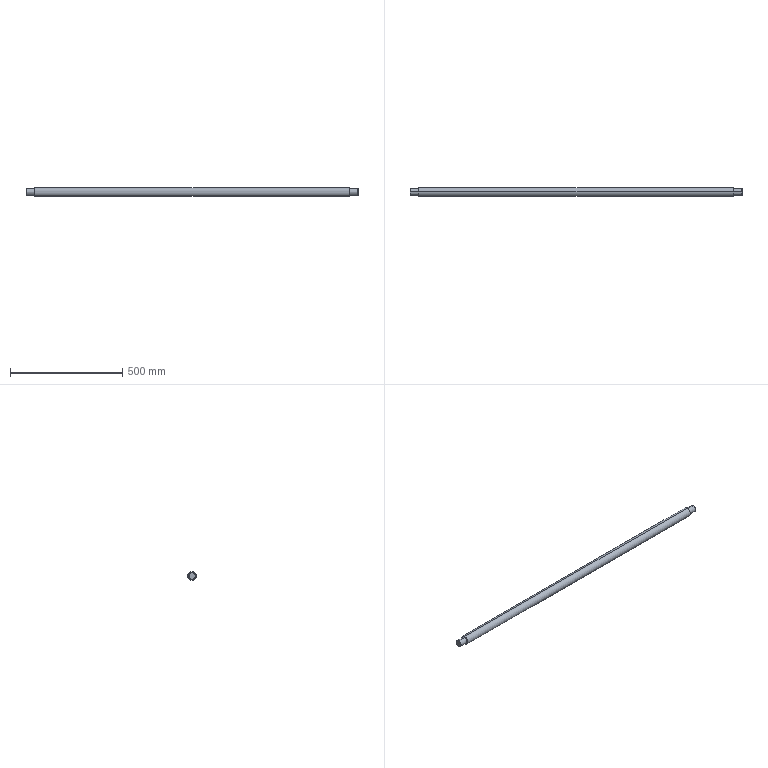Part | SolidWorks | features Chamfer 1, ICE 1, MirrorPattern 1, Revolution 1 | 1 solid | 29 faces | box 1476 x 40 x 40 mm | volume 1810594 mm3 | cone 10 | plane 10 | cylinder 9 | commonest cylinder face diameters 30 x4 8 x3 40 x2
STEP:
#1=CARTESIAN_POINT('',(-700.,0.,19.));
#2=VERTEX_POINT('',#1);
#3=CARTESIAN_POINT('',(-700.,0.,-19.));
#4=VERTEX_POINT('',#3);
#5=CARTESIAN_POINT('',(-700.,0.,0.));
#6=DIRECTION('',(-1.,0.,0.));
#7=DIRECTION('',(0.,0.,1.));
#8=AXIS2_PLACEMENT_3D('',#5,#6,#7);
#9=CIRCLE('',#8,19.);
#10=EDGE_CURVE('',#2,#4,#9,.T.);
#11=ORIENTED_EDGE('',*,*,#10,.F.);
#12=CARTESIAN_POINT('',(-699.,0.,20.));
#13=VERTEX_POINT('',#12);
#14=CARTESIAN_POINT('',(-699.,0.,20.));
#15=DIRECTION('',(0.7071,0.,0.7071));
#16=VECTOR('',#15,1000.);
#17=LINE('',#14,#16);
#18=EDGE_CURVE('',#2,#13,#17,.T.);
#19=ORIENTED_EDGE('',*,*,#18,.T.);
#20=CARTESIAN_POINT('',(-699.,0.,-20.));
#21=VERTEX_POINT('',#20);
#22=CARTESIAN_POINT('',(-699.,0.,0.));
#23=DIRECTION('',(1.,0.,0.));
#24=DIRECTION('',(0.,0.,1.));
#25=AXIS2_PLACEMENT_3D('',#22,#23,#24);
#26=CIRCLE('',#25,20.);
#27=EDGE_CURVE('',#21,#13,#26,.T.);
#28=ORIENTED_EDGE('',*,*,#27,.F.);
#29=CARTESIAN_POINT('',(-699.,0.,-20.));
#30=DIRECTION('',(0.7071,0.,-0.7071));
#31=VECTOR('',#30,1000.);
#32=LINE('',#29,#31);
#33=EDGE_CURVE('',#4,#21,#32,.T.);
#34=ORIENTED_EDGE('',*,*,#33,.F.);
#35=EDGE_LOOP('',(#11,#19,#28,#34));
#36=FACE_OUTER_BOUND('',#35,.T.);
#37=CARTESIAN_POINT('',(-699.,0.,0.));
#38=DIRECTION('',(1.,0.,0.));
#39=DIRECTION('',(0.,0.,-1.));
#40=AXIS2_PLACEMENT_3D('',#37,#38,#39);
#41=CONICAL_SURFACE('',#40,20.,0.7854);
#42=ADVANCED_FACE('',(#36),#41,.T.);
#43=CARTESIAN_POINT('',(-738.,0.,14.));
#44=VERTEX_POINT('',#43);
#45=CARTESIAN_POINT('',(-738.,13.416,4.));
#46=VERTEX_POINT('',#45);
#47=CARTESIAN_POINT('',(-738.,0.,0.));
#48=DIRECTION('',(-1.,0.,0.));
#49=DIRECTION('',(0.,0.,1.));
#50=AXIS2_PLACEMENT_3D('',#47,#48,#49);
#51=CIRCLE('',#50,14.);
#52=EDGE_CURVE('',#44,#46,#51,.T.);
#53=ORIENTED_EDGE('',*,*,#52,.F.);
#54=CARTESIAN_POINT('',(-737.,0.,15.));
#55=VERTEX_POINT('',#54);
#56=CARTESIAN_POINT('',(-737.,0.,15.));
#57=DIRECTION('',(0.7071,0.,0.7071));
#58=VECTOR('',#57,1000.);
#59=LINE('',#56,#58);
#60=EDGE_CURVE('',#44,#55,#59,.T.);
#61=ORIENTED_EDGE('',*,*,#60,.T.);
#62=CARTESIAN_POINT('',(-737.,14.457,4.));
#63=VERTEX_POINT('',#62);
#64=CARTESIAN_POINT('',(-737.,0.,0.));
#65=DIRECTION('',(1.,0.,0.));
#66=DIRECTION('',(0.,0.,1.));
#67=AXIS2_PLACEMENT_3D('',#64,#65,#66);
#68=CIRCLE('',#67,15.);
#69=EDGE_CURVE('',#63,#55,#68,.T.);
#70=ORIENTED_EDGE('',*,*,#69,.F.);
#71=CARTESIAN_POINT('',(-738.,13.416,4.));
#72=CARTESIAN_POINT('',(-737.667,13.764,4.));
#73=CARTESIAN_POINT('',(-737.334,14.11,4.));
#74=CARTESIAN_POINT('',(-737.,14.457,4.));
#75=B_SPLINE_CURVE_WITH_KNOTS('',3,(#71,#72,#73,#74),.UNSPECIFIED.,.F.,.F.,(4,4),(0.,0.001443),.UNSPECIFIED.);
#76=EDGE_CURVE('',#46,#63,#75,.T.);
#77=ORIENTED_EDGE('',*,*,#76,.F.);
#78=EDGE_LOOP('',(#53,#61,#70,#77));
#79=FACE_OUTER_BOUND('',#78,.T.);
#80=CARTESIAN_POINT('',(-737.,0.,0.));
#81=DIRECTION('',(1.,0.,0.));
#82=DIRECTION('',(0.,0.,-1.));
#83=AXIS2_PLACEMENT_3D('',#80,#81,#82);
#84=CONICAL_SURFACE('',#83,15.,0.7854);
#85=ADVANCED_FACE('',(#79),#84,.T.);
#86=ORIENTED_EDGE('',*,*,#60,.F.);
#87=CARTESIAN_POINT('',(-738.,0.,-14.));
#88=VERTEX_POINT('',#87);
#89=CARTESIAN_POINT('',(-738.,0.,0.));
#90=DIRECTION('',(-1.,0.,0.));
#91=DIRECTION('',(0.,0.,1.));
#92=AXIS2_PLACEMENT_3D('',#89,#90,#91);
#93=CIRCLE('',#92,14.);
#94=EDGE_CURVE('',#88,#44,#93,.T.);
#95=ORIENTED_EDGE('',*,*,#94,.F.);
#96=CARTESIAN_POINT('',(-737.,0.,-15.));
#97=VERTEX_POINT('',#96);
#98=CARTESIAN_POINT('',(-737.,0.,-15.));
#99=DIRECTION('',(0.7071,0.,-0.7071));
#100=VECTOR('',#99,1000.);
#101=LINE('',#98,#100);
#102=EDGE_CURVE('',#88,#97,#101,.T.);
#103=ORIENTED_EDGE('',*,*,#102,.T.);
#104=CARTESIAN_POINT('',(-737.,0.,0.));
#105=DIRECTION('',(1.,0.,0.));
#106=DIRECTION('',(0.,0.,1.));
#107=AXIS2_PLACEMENT_3D('',#104,#105,#106);
#108=CIRCLE('',#107,15.);
#109=EDGE_CURVE('',#55,#97,#108,.T.);
#110=ORIENTED_EDGE('',*,*,#109,.F.);
#111=EDGE_LOOP('',(#86,#95,#103,#110));
#112=FACE_OUTER_BOUND('',#111,.T.);
#113=CARTESIAN_POINT('',(-737.,0.,0.));
#114=DIRECTION('',(1.,0.,0.));
#115=DIRECTION('',(0.,0.,-1.));
#116=AXIS2_PLACEMENT_3D('',#113,#114,#115);
#117=CONICAL_SURFACE('',#116,15.,0.7854);
#118=ADVANCED_FACE('',(#112),#117,.T.);
#119=CARTESIAN_POINT('',(700.,0.,-19.));
#120=VERTEX_POINT('',#119);
#121=CARTESIAN_POINT('',(700.,0.,19.));
#122=VERTEX_POINT('',#121);
#123=CARTESIAN_POINT('',(700.,0.,0.));
#124=DIRECTION('',(1.,0.,0.));
#125=DIRECTION('',(0.,0.,-1.));
#126=AXIS2_PLACEMENT_3D('',#123,#124,#125);
#127=CIRCLE('',#126,19.);
#128=EDGE_CURVE('',#120,#122,#127,.T.);
#129=ORIENTED_EDGE('',*,*,#128,.F.);
#130=CARTESIAN_POINT('',(699.,0.,-20.));
#131=VERTEX_POINT('',#130);
#132=CARTESIAN_POINT('',(700.,0.,-19.));
#133=DIRECTION('',(-0.7071,0.,-0.7071));
#134=VECTOR('',#133,1000.);
#135=LINE('',#132,#134);
#136=EDGE_CURVE('',#120,#131,#135,.T.);
#137=ORIENTED_EDGE('',*,*,#136,.T.);
#138=CARTESIAN_POINT('',(699.,0.,20.));
#139=VERTEX_POINT('',#138);
#140=CARTESIAN_POINT('',(699.,0.,0.));
#141=DIRECTION('',(-1.,0.,0.));
#142=DIRECTION('',(0.,0.,-1.));
#143=AXIS2_PLACEMENT_3D('',#140,#141,#142);
#144=CIRCLE('',#143,20.);
#145=EDGE_CURVE('',#139,#131,#144,.T.);
#146=ORIENTED_EDGE('',*,*,#145,.F.);
#147=CARTESIAN_POINT('',(700.,0.,19.));
#148=DIRECTION('',(-0.7071,0.,0.7071));
#149=VECTOR('',#148,1000.);
#150=LINE('',#147,#149);
#151=EDGE_CURVE('',#122,#139,#150,.T.);
#152=ORIENTED_EDGE('',*,*,#151,.F.);
#153=EDGE_LOOP('',(#129,#137,#146,#152));
#154=FACE_OUTER_BOUND('',#153,.T.);
#155=CARTESIAN_POINT('',(700.,0.,0.));
#156=DIRECTION('',(-1.,0.,0.));
#157=DIRECTION('',(0.,0.,1.));
#158=AXIS2_PLACEMENT_3D('',#155,#156,#157);
#159=CONICAL_SURFACE('',#158,19.,0.7854);
#160=ADVANCED_FACE('',(#154),#159,.T.);
#161=CARTESIAN_POINT('',(738.,0.,-14.));
#162=VERTEX_POINT('',#161);
#163=CARTESIAN_POINT('',(738.,13.416,-4.));
#164=VERTEX_POINT('',#163);
#165=CARTESIAN_POINT('',(738.,0.,0.));
#166=DIRECTION('',(1.,0.,0.));
#167=DIRECTION('',(0.,0.,-1.));
#168=AXIS2_PLACEMENT_3D('',#165,#166,#167);
#169=CIRCLE('',#168,14.);
#170=EDGE_CURVE('',#162,#164,#169,.T.);
#171=ORIENTED_EDGE('',*,*,#170,.F.);
#172=CARTESIAN_POINT('',(737.,0.,-15.));
#173=VERTEX_POINT('',#172);
#174=CARTESIAN_POINT('',(738.,0.,-14.));
#175=DIRECTION('',(-0.7071,0.,-0.7071));
#176=VECTOR('',#175,1000.);
#177=LINE('',#174,#176);
#178=EDGE_CURVE('',#162,#173,#177,.T.);
#179=ORIENTED_EDGE('',*,*,#178,.T.);
#180=CARTESIAN_POINT('',(737.,14.457,-4.));
#181=VERTEX_POINT('',#180);
#182=CARTESIAN_POINT('',(737.,0.,0.));
#183=DIRECTION('',(-1.,0.,0.));
#184=DIRECTION('',(0.,0.,-1.));
#185=AXIS2_PLACEMENT_3D('',#182,#183,#184);
#186=CIRCLE('',#185,15.);
#187=EDGE_CURVE('',#181,#173,#186,.T.);
#188=ORIENTED_EDGE('',*,*,#187,.F.);
#189=CARTESIAN_POINT('',(738.,13.416,-4.));
#190=CARTESIAN_POINT('',(737.667,13.764,-4.));
#191=CARTESIAN_POINT('',(737.334,14.11,-4.));
#192=CARTESIAN_POINT('',(737.,14.457,-4.));
#193=B_SPLINE_CURVE_WITH_KNOTS('',3,(#189,#190,#191,#192),.UNSPECIFIED.,.F.,.F.,(4,4),(0.,0.001443),.UNSPECIFIED.);
#194=EDGE_CURVE('',#164,#181,#193,.T.);
#195=ORIENTED_EDGE('',*,*,#194,.F.);
#196=EDGE_LOOP('',(#171,#179,#188,#195));
#197=FACE_OUTER_BOUND('',#196,.T.);
#198=CARTESIAN_POINT('',(738.,0.,0.));
#199=DIRECTION('',(-1.,0.,0.));
#200=DIRECTION('',(0.,0.,1.));
#201=AXIS2_PLACEMENT_3D('',#198,#199,#200);
#202=CONICAL_SURFACE('',#201,14.,0.7854);
#203=ADVANCED_FACE('',(#197),#202,.T.);
#204=ORIENTED_EDGE('',*,*,#178,.F.);
#205=CARTESIAN_POINT('',(738.,0.,14.));
#206=VERTEX_POINT('',#205);
#207=CARTESIAN_POINT('',(738.,0.,0.));
#208=DIRECTION('',(1.,0.,0.));
#209=DIRECTION('',(0.,0.,-1.));
#210=AXIS2_PLACEMENT_3D('',#207,#208,#209);
#211=CIRCLE('',#210,14.);
#212=EDGE_CURVE('',#206,#162,#211,.T.);
#213=ORIENTED_EDGE('',*,*,#212,.F.);
#214=CARTESIAN_POINT('',(737.,0.,15.));
#215=VERTEX_POINT('',#214);
#216=CARTESIAN_POINT('',(738.,0.,14.));
#217=DIRECTION('',(-0.7071,0.,0.7071));
#218=VECTOR('',#217,1000.);
#219=LINE('',#216,#218);
#220=EDGE_CURVE('',#206,#215,#219,.T.);
#221=ORIENTED_EDGE('',*,*,#220,.T.);
#222=CARTESIAN_POINT('',(737.,0.,0.));
#223=DIRECTION('',(-1.,0.,0.));
#224=DIRECTION('',(0.,0.,-1.));
#225=AXIS2_PLACEMENT_3D('',#222,#223,#224);
#226=CIRCLE('',#225,15.);
#227=EDGE_CURVE('',#173,#215,#226,.T.);
#228=ORIENTED_EDGE('',*,*,#227,.F.);
#229=EDGE_LOOP('',(#204,#213,#221,#228));
#230=FACE_OUTER_BOUND('',#229,.T.);
#231=CARTESIAN_POINT('',(738.,0.,0.));
#232=DIRECTION('',(-1.,0.,0.));
#233=DIRECTION('',(0.,0.,1.));
#234=AXIS2_PLACEMENT_3D('',#231,#232,#233);
#235=CONICAL_SURFACE('',#234,14.,0.7854);
#236=ADVANCED_FACE('',(#230),#235,.T.);
#237=CARTESIAN_POINT('',(705.,11.,4.));
#238=VERTEX_POINT('',#237);
#239=CARTESIAN_POINT('',(701.,11.,0.));
#240=VERTEX_POINT('',#239);
#241=CARTESIAN_POINT('',(705.,11.,0.));
#242=DIRECTION('',(0.,-1.,0.));
#243=DIRECTION('',(1.,0.,0.));
#244=AXIS2_PLACEMENT_3D('',#241,#242,#243);
#245=CIRCLE('',#244,4.);
#246=EDGE_CURVE('',#238,#240,#245,.T.);
#247=ORIENTED_EDGE('',*,*,#246,.T.);
#248=CARTESIAN_POINT('',(701.,15.,0.));
#249=VERTEX_POINT('',#248);
#250=CARTESIAN_POINT('',(701.,11.,0.));
#251=DIRECTION('',(0.,1.,0.));
#252=VECTOR('',#251,1000.);
#253=LINE('',#250,#252);
#254=EDGE_CURVE('',#240,#249,#253,.T.);
#255=ORIENTED_EDGE('',*,*,#254,.T.);
#256=CARTESIAN_POINT('',(705.,14.457,4.));
#257=VERTEX_POINT('',#256);
#258=CARTESIAN_POINT('',(705.,14.457,4.));
#259=CARTESIAN_POINT('',(704.734,14.457,4.));
#260=CARTESIAN_POINT('',(704.473,14.464,3.974));
#261=CARTESIAN_POINT('',(703.96,14.492,3.871));
#262=CARTESIAN_POINT('',(703.706,14.513,3.794));
#263=CARTESIAN_POINT('',(703.222,14.564,3.593));
#264=CARTESIAN_POINT('',(702.992,14.594,3.47));
#265=CARTESIAN_POINT('',(702.558,14.66,3.179));
#266=CARTESIAN_POINT('',(702.354,14.696,3.011));
#267=CARTESIAN_POINT('',(701.987,14.766,2.644));
#268=CARTESIAN_POINT('',(701.822,14.801,2.443));
#269=CARTESIAN_POINT('',(701.529,14.867,2.006));
#270=CARTESIAN_POINT('',(701.406,14.897,1.775));
#271=CARTESIAN_POINT('',(701.206,14.946,1.293));
#272=CARTESIAN_POINT('',(701.129,14.966,1.04));
#273=CARTESIAN_POINT('',(701.026,14.993,0.5228));
#274=CARTESIAN_POINT('',(701.,15.,0.2623));
#275=CARTESIAN_POINT('',(701.,15.,0.));
#276=B_SPLINE_CURVE_WITH_KNOTS('',3,(#258,#259,#260,#261,#262,#263,#264,#265,#266,#267,#268,#269,#270,#271,#272,#273,#274,#275),.UNSPECIFIED.,.F.,.F.,(4,2,2,2,2,2,2,2,4),(0.,0.0007854,0.001571,0.002356,0.003142,0.003927,0.004712,0.005498,0.006283),.UNSPECIFIED.);
#277=EDGE_CURVE('',#257,#249,#276,.T.);
#278=ORIENTED_EDGE('',*,*,#277,.F.);
#279=CARTESIAN_POINT('',(705.,11.,4.));
#280=DIRECTION('',(0.,1.,0.));
#281=VECTOR('',#280,1000.);
#282=LINE('',#279,#281);
#283=EDGE_CURVE('',#238,#257,#282,.T.);
#284=ORIENTED_EDGE('',*,*,#283,.F.);
#285=EDGE_LOOP('',(#247,#255,#278,#284));
#286=FACE_OUTER_BOUND('',#285,.T.);
#287=CARTESIAN_POINT('',(705.,11.,0.));
#288=DIRECTION('',(0.,1.,0.));
#289=DIRECTION('',(-1.,0.,0.));
#290=AXIS2_PLACEMENT_3D('',#287,#288,#289);
#291=CYLINDRICAL_SURFACE('',#290,4.);
#292=ADVANCED_FACE('',(#286),#291,.F.);
#293=ORIENTED_EDGE('',*,*,#27,.T.);
#294=CARTESIAN_POINT('',(738.,0.,20.));
#295=DIRECTION('',(1.,0.,0.));
#296=VECTOR('',#295,1000.);
#297=LINE('',#294,#296);
#298=EDGE_CURVE('',#13,#139,#297,.T.);
#299=ORIENTED_EDGE('',*,*,#298,.T.);
#300=ORIENTED_EDGE('',*,*,#145,.T.);
#301=CARTESIAN_POINT('',(738.,0.,-20.));
#302=DIRECTION('',(1.,0.,0.));
#303=VECTOR('',#302,1000.);
#304=LINE('',#301,#303);
#305=EDGE_CURVE('',#21,#131,#304,.T.);
#306=ORIENTED_EDGE('',*,*,#305,.F.);
#307=EDGE_LOOP('',(#293,#299,#300,#306));
#308=FACE_OUTER_BOUND('',#307,.T.);
#309=CARTESIAN_POINT('',(738.,0.,0.));
#310=DIRECTION('',(1.,0.,0.));
#311=DIRECTION('',(0.,0.,-1.));
#312=AXIS2_PLACEMENT_3D('',#309,#310,#311);
#313=CYLINDRICAL_SURFACE('',#312,20.);
#314=ADVANCED_FACE('',(#308),#313,.T.);
#315=ORIENTED_EDGE('',*,*,#69,.T.);
#316=CARTESIAN_POINT('',(-700.,0.,15.));
#317=VERTEX_POINT('',#316);
#318=CARTESIAN_POINT('',(738.,0.,15.));
#319=DIRECTION('',(1.,0.,0.));
#320=VECTOR('',#319,1000.);
#321=LINE('',#318,#320);
#322=EDGE_CURVE('',#55,#317,#321,.T.);
#323=ORIENTED_EDGE('',*,*,#322,.T.);
#324=CARTESIAN_POINT('',(-700.,0.,-15.));
#325=VERTEX_POINT('',#324);
#326=CARTESIAN_POINT('',(-700.,0.,0.));
#327=DIRECTION('',(1.,0.,0.));
#328=DIRECTION('',(0.,0.,-1.));
#329=AXIS2_PLACEMENT_3D('',#326,#327,#328);
#330=CIRCLE('',#329,15.);
#331=EDGE_CURVE('',#325,#317,#330,.T.);
#332=ORIENTED_EDGE('',*,*,#331,.F.);
#333=CARTESIAN_POINT('',(738.,0.,-15.));
#334=DIRECTION('',(1.,0.,0.));
#335=VECTOR('',#334,1000.);
#336=LINE('',#333,#335);
#337=EDGE_CURVE('',#97,#325,#336,.T.);
#338=ORIENTED_EDGE('',*,*,#337,.F.);
#339=CARTESIAN_POINT('',(-737.,14.457,-4.));
#340=VERTEX_POINT('',#339);
#341=CARTESIAN_POINT('',(-737.,0.,0.));
#342=DIRECTION('',(1.,0.,0.));
#343=DIRECTION('',(0.,0.,1.));
#344=AXIS2_PLACEMENT_3D('',#341,#342,#343);
#345=CIRCLE('',#344,15.);
#346=EDGE_CURVE('',#97,#340,#345,.T.);
#347=ORIENTED_EDGE('',*,*,#346,.T.);
#348=CARTESIAN_POINT('',(-705.,14.457,-4.));
#349=VERTEX_POINT('',#348);
#350=CARTESIAN_POINT('',(738.,14.457,-4.));
#351=DIRECTION('',(-1.,0.,0.));
#352=VECTOR('',#351,1000.);
#353=LINE('',#350,#352);
#354=EDGE_CURVE('',#349,#340,#353,.T.);
#355=ORIENTED_EDGE('',*,*,#354,.F.);
#356=CARTESIAN_POINT('',(-705.,14.457,4.));
#357=VERTEX_POINT('',#356);
#358=CARTESIAN_POINT('',(-705.,14.457,4.));
#359=CARTESIAN_POINT('',(-704.734,14.457,4.));
#360=CARTESIAN_POINT('',(-704.474,14.464,3.974));
#361=CARTESIAN_POINT('',(-703.961,14.492,3.872));
#362=CARTESIAN_POINT('',(-703.706,14.513,3.794));
#363=CARTESIAN_POINT('',(-703.223,14.564,3.593));
#364=CARTESIAN_POINT('',(-702.993,14.594,3.47));
#365=CARTESIAN_POINT('',(-702.56,14.66,3.18));
#366=CARTESIAN_POINT('',(-702.355,14.696,3.012));
#367=CARTESIAN_POINT('',(-701.988,14.766,2.645));
#368=CARTESIAN_POINT('',(-701.823,14.801,2.444));
#369=CARTESIAN_POINT('',(-701.53,14.867,2.008));
#370=CARTESIAN_POINT('',(-701.407,14.896,1.777));
#371=CARTESIAN_POINT('',(-701.207,14.946,1.296));
#372=CARTESIAN_POINT('',(-701.129,14.966,1.043));
#373=CARTESIAN_POINT('',(-701.026,14.993,0.5261));
#374=CARTESIAN_POINT('',(-701.,15.,0.2658));
#375=CARTESIAN_POINT('',(-701.,15.,-0.2585));
#376=CARTESIAN_POINT('',(-701.026,14.993,-0.5249));
#377=CARTESIAN_POINT('',(-701.128,14.966,-1.039));
#378=CARTESIAN_POINT('',(-701.204,14.947,-1.289));
#379=CARTESIAN_POINT('',(-701.506,14.872,-2.017));
#380=CARTESIAN_POINT('',(-701.801,14.802,-2.457));
#381=CARTESIAN_POINT('',(-702.355,14.696,-3.012));
#382=CARTESIAN_POINT('',(-702.556,14.66,-3.177));
#383=CARTESIAN_POINT('',(-702.988,14.595,-3.467));
#384=CARTESIAN_POINT('',(-703.222,14.564,-3.593));
#385=CARTESIAN_POINT('',(-703.704,14.513,-3.793));
#386=CARTESIAN_POINT('',(-703.954,14.492,-3.87));
#387=CARTESIAN_POINT('',(-704.469,14.464,-3.973));
#388=CARTESIAN_POINT('',(-704.734,14.457,-4.));
#389=CARTESIAN_POINT('',(-705.,14.457,-4.));
#390=B_SPLINE_CURVE_WITH_KNOTS('',3,(#358,#359,#360,#361,#362,#363,#364,#365,#366,#367,#368,#369,#370,#371,#372,#373,#374,#375,#376,#377,#378,#379,#380,#381,#382,#383,#384,#385,#386,#387,#388,#389),.UNSPECIFIED.,.F.,.F.,(4,2,2,2,2,2,2,2,2,2,2,2,2,2,2,4),(0.,0.0007849,0.00157,0.002355,0.00314,0.003925,0.00471,0.005494,0.006279,0.007064,0.007849,0.009419,0.0102,0.01099,0.01177,0.01256),.UNSPECIFIED.);
#391=EDGE_CURVE('',#357,#349,#390,.T.);
#392=ORIENTED_EDGE('',*,*,#391,.F.);
#393=CARTESIAN_POINT('',(738.,14.457,4.));
#394=DIRECTION('',(1.,0.,0.));
#395=VECTOR('',#394,1000.);
#396=LINE('',#393,#395);
#397=EDGE_CURVE('',#63,#357,#396,.T.);
#398=ORIENTED_EDGE('',*,*,#397,.F.);
#399=EDGE_LOOP('',(#315,#323,#332,#338,#347,#355,#392,#398));
#400=FACE_OUTER_BOUND('',#399,.T.);
#401=CARTESIAN_POINT('',(738.,0.,0.));
#402=DIRECTION('',(1.,0.,0.));
#403=DIRECTION('',(0.,0.,-1.));
#404=AXIS2_PLACEMENT_3D('',#401,#402,#403);
#405=CYLINDRICAL_SURFACE('',#404,15.);
#406=ADVANCED_FACE('',(#400),#405,.T.);
#407=CARTESIAN_POINT('',(700.,0.,-15.));
#408=VERTEX_POINT('',#407);
#409=CARTESIAN_POINT('',(700.,0.,15.));
#410=VERTEX_POINT('',#409);
#411=CARTESIAN_POINT('',(700.,0.,0.));
#412=DIRECTION('',(1.,0.,0.));
#413=DIRECTION('',(0.,0.,-1.));
#414=AXIS2_PLACEMENT_3D('',#411,#412,#413);
#415=CIRCLE('',#414,15.);
#416=EDGE_CURVE('',#408,#410,#415,.T.);
#417=ORIENTED_EDGE('',*,*,#416,.T.);
#418=CARTESIAN_POINT('',(738.,0.,15.));
#419=DIRECTION('',(1.,0.,0.));
#420=VECTOR('',#419,1000.);
#421=LINE('',#418,#420);
#422=EDGE_CURVE('',#410,#215,#421,.T.);
#423=ORIENTED_EDGE('',*,*,#422,.T.);
#424=CARTESIAN_POINT('',(737.,14.457,4.));
#425=VERTEX_POINT('',#424);
#426=CARTESIAN_POINT('',(737.,0.,0.));
#427=DIRECTION('',(-1.,0.,0.));
#428=DIRECTION('',(0.,0.,-1.));
#429=AXIS2_PLACEMENT_3D('',#426,#427,#428);
#430=CIRCLE('',#429,15.);
#431=EDGE_CURVE('',#215,#425,#430,.T.);
#432=ORIENTED_EDGE('',*,*,#431,.T.);
#433=CARTESIAN_POINT('',(738.,14.457,4.));
#434=DIRECTION('',(-1.,0.,0.));
#435=VECTOR('',#434,1000.);
#436=LINE('',#433,#435);
#437=EDGE_CURVE('',#425,#257,#436,.T.);
#438=ORIENTED_EDGE('',*,*,#437,.T.);
#439=ORIENTED_EDGE('',*,*,#277,.T.);
#440=CARTESIAN_POINT('',(705.,14.457,-4.));
#441=VERTEX_POINT('',#440);
#442=CARTESIAN_POINT('',(701.,15.,0.));
#443=CARTESIAN_POINT('',(701.,15.,-0.262));
#444=CARTESIAN_POINT('',(701.026,14.993,-0.5282));
#445=CARTESIAN_POINT('',(701.129,14.966,-1.042));
#446=CARTESIAN_POINT('',(701.205,14.946,-1.292));
#447=CARTESIAN_POINT('',(701.508,14.871,-2.02));
#448=CARTESIAN_POINT('',(701.802,14.802,-2.459));
#449=CARTESIAN_POINT('',(702.357,14.695,-3.014));
#450=CARTESIAN_POINT('',(702.557,14.66,-3.178));
#451=CARTESIAN_POINT('',(702.989,14.594,-3.467));
#452=CARTESIAN_POINT('',(703.223,14.564,-3.593));
#453=CARTESIAN_POINT('',(703.705,14.513,-3.794));
#454=CARTESIAN_POINT('',(703.954,14.492,-3.87));
#455=CARTESIAN_POINT('',(704.469,14.464,-3.973));
#456=CARTESIAN_POINT('',(704.735,14.457,-4.));
#457=CARTESIAN_POINT('',(705.,14.457,-4.));
#458=B_SPLINE_CURVE_WITH_KNOTS('',3,(#442,#443,#444,#445,#446,#447,#448,#449,#450,#451,#452,#453,#454,#455,#456,#457),.UNSPECIFIED.,.F.,.F.,(4,2,2,2,2,2,2,4),(0.006283,0.007068,0.007852,0.009421,0.01021,0.01099,0.01177,0.01256),.UNSPECIFIED.);
#459=EDGE_CURVE('',#249,#441,#458,.T.);
#460=ORIENTED_EDGE('',*,*,#459,.T.);
#461=CARTESIAN_POINT('',(738.,14.457,-4.));
#462=DIRECTION('',(1.,0.,0.));
#463=VECTOR('',#462,1000.);
#464=LINE('',#461,#463);
#465=EDGE_CURVE('',#441,#181,#464,.T.);
#466=ORIENTED_EDGE('',*,*,#465,.T.);
#467=ORIENTED_EDGE('',*,*,#187,.T.);
#468=CARTESIAN_POINT('',(738.,0.,-15.));
#469=DIRECTION('',(1.,0.,0.));
#470=VECTOR('',#469,1000.);
#471=LINE('',#468,#470);
#472=EDGE_CURVE('',#408,#173,#471,.T.);
#473=ORIENTED_EDGE('',*,*,#472,.F.);
#474=EDGE_LOOP('',(#417,#423,#432,#438,#439,#460,#466,#467,#473));
#475=FACE_OUTER_BOUND('',#474,.T.);
#476=CARTESIAN_POINT('',(738.,0.,0.));
#477=DIRECTION('',(1.,0.,0.));
#478=DIRECTION('',(0.,0.,-1.));
#479=AXIS2_PLACEMENT_3D('',#476,#477,#478);
#480=CYLINDRICAL_SURFACE('',#479,15.);
#481=ADVANCED_FACE('',(#475),#480,.T.);
#482=ORIENTED_EDGE('',*,*,#422,.F.);
#483=CARTESIAN_POINT('',(700.,0.,0.));
#484=DIRECTION('',(1.,0.,0.));
#485=DIRECTION('',(0.,0.,-1.));
#486=AXIS2_PLACEMENT_3D('',#483,#484,#485);
#487=CIRCLE('',#486,15.);
#488=EDGE_CURVE('',#410,#408,#487,.T.);
#489=ORIENTED_EDGE('',*,*,#488,.T.);
#490=ORIENTED_EDGE('',*,*,#472,.T.);
#491=ORIENTED_EDGE('',*,*,#227,.T.);
#492=EDGE_LOOP('',(#482,#489,#490,#491));
#493=FACE_OUTER_BOUND('',#492,.T.);
#494=CARTESIAN_POINT('',(738.,0.,0.));
#495=DIRECTION('',(1.,0.,0.));
#496=DIRECTION('',(0.,0.,-1.));
#497=AXIS2_PLACEMENT_3D('',#494,#495,#496);
#498=CYLINDRICAL_SURFACE('',#497,15.);
#499=ADVANCED_FACE('',(#493),#498,.T.);
#500=CARTESIAN_POINT('',(738.,11.,4.));
#501=VERTEX_POINT('',#500);
#502=CARTESIAN_POINT('',(738.,13.416,4.));
#503=VERTEX_POINT('',#502);
#504=CARTESIAN_POINT('',(738.,11.,4.));
#505=DIRECTION('',(0.,1.,0.));
#506=VECTOR('',#505,1000.);
#507=LINE('',#504,#506);
#508=EDGE_CURVE('',#501,#503,#507,.T.);
#509=ORIENTED_EDGE('',*,*,#508,.T.);
#510=CARTESIAN_POINT('',(738.,0.,0.));
#511=DIRECTION('',(1.,0.,0.));
#512=DIRECTION('',(0.,0.,-1.));
#513=AXIS2_PLACEMENT_3D('',#510,#511,#512);
#514=CIRCLE('',#513,14.);
#515=EDGE_CURVE('',#503,#206,#514,.T.);
#516=ORIENTED_EDGE('',*,*,#515,.T.);
#517=ORIENTED_EDGE('',*,*,#212,.T.);
#518=ORIENTED_EDGE('',*,*,#170,.T.);
#519=CARTESIAN_POINT('',(738.,11.,-4.));
#520=VERTEX_POINT('',#519);
#521=CARTESIAN_POINT('',(738.,11.,-4.));
#522=DIRECTION('',(0.,1.,0.));
#523=VECTOR('',#522,1000.);
#524=LINE('',#521,#523);
#525=EDGE_CURVE('',#520,#164,#524,.T.);
#526=ORIENTED_EDGE('',*,*,#525,.F.);
#527=CARTESIAN_POINT('',(738.,11.,-4.));
#528=DIRECTION('',(0.,0.,1.));
#529=VECTOR('',#528,1000.);
#530=LINE('',#527,#529);
#531=EDGE_CURVE('',#520,#501,#530,.T.);
#532=ORIENTED_EDGE('',*,*,#531,.T.);
#533=EDGE_LOOP('',(#509,#516,#517,#518,#526,#532));
#534=FACE_OUTER_BOUND('',#533,.T.);
#535=CARTESIAN_POINT('',(738.,15.,0.));
#536=DIRECTION('',(1.,0.,0.));
#537=DIRECTION('',(0.,0.,-1.));
#538=AXIS2_PLACEMENT_3D('',#535,#536,#537);
#539=PLANE('',#538);
#540=ADVANCED_FACE('',(#534),#539,.T.);
#541=CARTESIAN_POINT('',(-738.,11.,-4.));
#542=VERTEX_POINT('',#541);
#543=CARTESIAN_POINT('',(-738.,13.416,-4.));
#544=VERTEX_POINT('',#543);
#545=CARTESIAN_POINT('',(-738.,11.,-4.));
#546=DIRECTION('',(0.,1.,0.));
#547=VECTOR('',#546,1000.);
#548=LINE('',#545,#547);
#549=EDGE_CURVE('',#542,#544,#548,.T.);
#550=ORIENTED_EDGE('',*,*,#549,.T.);
#551=CARTESIAN_POINT('',(-738.,0.,0.));
#552=DIRECTION('',(-1.,0.,0.));
#553=DIRECTION('',(0.,0.,1.));
#554=AXIS2_PLACEMENT_3D('',#551,#552,#553);
#555=CIRCLE('',#554,14.);
#556=EDGE_CURVE('',#544,#88,#555,.T.);
#557=ORIENTED_EDGE('',*,*,#556,.T.);
#558=ORIENTED_EDGE('',*,*,#94,.T.);
#559=ORIENTED_EDGE('',*,*,#52,.T.);
#560=CARTESIAN_POINT('',(-738.,11.,4.));
#561=VERTEX_POINT('',#560);
#562=CARTESIAN_POINT('',(-738.,11.,4.));
#563=DIRECTION('',(0.,1.,0.));
#564=VECTOR('',#563,1000.);
#565=LINE('',#562,#564);
#566=EDGE_CURVE('',#561,#46,#565,.T.);
#567=ORIENTED_EDGE('',*,*,#566,.F.);
#568=CARTESIAN_POINT('',(-738.,11.,-4.));
#569=DIRECTION('',(0.,0.,1.));
#570=VECTOR('',#569,1000.);
#571=LINE('',#568,#570);
#572=EDGE_CURVE('',#542,#561,#571,.T.);
#573=ORIENTED_EDGE('',*,*,#572,.F.);
#574=EDGE_LOOP('',(#550,#557,#558,#559,#567,#573));
#575=FACE_OUTER_BOUND('',#574,.T.);
#576=CARTESIAN_POINT('',(-738.,0.,0.));
#577=DIRECTION('',(-1.,0.,0.));
#578=DIRECTION('',(0.,0.,1.));
#579=AXIS2_PLACEMENT_3D('',#576,#577,#578);
#580=PLANE('',#579);
#581=ADVANCED_FACE('',(#575),#580,.T.);
#582=ORIENTED_EDGE('',*,*,#322,.F.);
#583=ORIENTED_EDGE('',*,*,#109,.T.);
#584=ORIENTED_EDGE('',*,*,#337,.T.);
#585=CARTESIAN_POINT('',(-700.,0.,0.));
#586=DIRECTION('',(1.,0.,0.));
#587=DIRECTION('',(0.,0.,-1.));
#588=AXIS2_PLACEMENT_3D('',#585,#586,#587);
#589=CIRCLE('',#588,15.);
#590=EDGE_CURVE('',#317,#325,#589,.T.);
#591=ORIENTED_EDGE('',*,*,#590,.F.);
#592=EDGE_LOOP('',(#582,#583,#584,#591));
#593=FACE_OUTER_BOUND('',#592,.T.);
#594=CARTESIAN_POINT('',(738.,0.,0.));
#595=DIRECTION('',(1.,0.,0.));
#596=DIRECTION('',(0.,0.,-1.));
#597=AXIS2_PLACEMENT_3D('',#594,#595,#596);
#598=CYLINDRICAL_SURFACE('',#597,15.);
#599=ADVANCED_FACE('',(#593),#598,.T.);
#600=CARTESIAN_POINT('',(-700.,0.,0.));
#601=DIRECTION('',(-1.,0.,0.));
#602=DIRECTION('',(0.,0.,1.));
#603=AXIS2_PLACEMENT_3D('',#600,#601,#602);
#604=CIRCLE('',#603,19.);
#605=EDGE_CURVE('',#4,#2,#604,.T.);
#606=ORIENTED_EDGE('',*,*,#605,.T.);
#607=ORIENTED_EDGE('',*,*,#10,.T.);
#608=EDGE_LOOP('',(#606,#607));
#609=FACE_OUTER_BOUND('',#608,.T.);
#610=ORIENTED_EDGE('',*,*,#331,.T.);
#611=ORIENTED_EDGE('',*,*,#590,.T.);
#612=EDGE_LOOP('',(#610,#611));
#613=FACE_BOUND('',#612,.T.);
#614=CARTESIAN_POINT('',(-700.,15.,0.));
#615=DIRECTION('',(-1.,0.,0.));
#616=DIRECTION('',(0.,0.,1.));
#617=AXIS2_PLACEMENT_3D('',#614,#615,#616);
#618=PLANE('',#617);
#619=ADVANCED_FACE('',(#609,#613),#618,.T.);
#620=ORIENTED_EDGE('',*,*,#298,.F.);
#621=CARTESIAN_POINT('',(-699.,0.,0.));
#622=DIRECTION('',(1.,0.,0.));
#623=DIRECTION('',(0.,0.,1.));
#624=AXIS2_PLACEMENT_3D('',#621,#622,#623);
#625=CIRCLE('',#624,20.);
#626=EDGE_CURVE('',#13,#21,#625,.T.);
#627=ORIENTED_EDGE('',*,*,#626,.T.);
#628=ORIENTED_EDGE('',*,*,#305,.T.);
#629=CARTESIAN_POINT('',(699.,0.,0.));
#630=DIRECTION('',(-1.,0.,0.));
#631=DIRECTION('',(0.,0.,-1.));
#632=AXIS2_PLACEMENT_3D('',#629,#630,#631);
#633=CIRCLE('',#632,20.);
#634=EDGE_CURVE('',#131,#139,#633,.T.);
#635=ORIENTED_EDGE('',*,*,#634,.T.);
#636=EDGE_LOOP('',(#620,#627,#628,#635));
#637=FACE_OUTER_BOUND('',#636,.T.);
#638=CARTESIAN_POINT('',(738.,0.,0.));
#639=DIRECTION('',(1.,0.,0.));
#640=DIRECTION('',(0.,0.,-1.));
#641=AXIS2_PLACEMENT_3D('',#638,#639,#640);
#642=CYLINDRICAL_SURFACE('',#641,20.);
#643=ADVANCED_FACE('',(#637),#642,.T.);
#644=CARTESIAN_POINT('',(700.,0.,0.));
#645=DIRECTION('',(1.,0.,0.));
#646=DIRECTION('',(0.,0.,-1.));
#647=AXIS2_PLACEMENT_3D('',#644,#645,#646);
#648=CIRCLE('',#647,19.);
#649=EDGE_CURVE('',#122,#120,#648,.T.);
#650=ORIENTED_EDGE('',*,*,#649,.T.);
#651=ORIENTED_EDGE('',*,*,#128,.T.);
#652=EDGE_LOOP('',(#650,#651));
#653=FACE_OUTER_BOUND('',#652,.T.);
#654=ORIENTED_EDGE('',*,*,#416,.F.);
#655=ORIENTED_EDGE('',*,*,#488,.F.);
#656=EDGE_LOOP('',(#654,#655));
#657=FACE_BOUND('',#656,.T.);
#658=CARTESIAN_POINT('',(700.,20.,0.));
#659=DIRECTION('',(1.,0.,0.));
#660=DIRECTION('',(0.,0.,-1.));
#661=AXIS2_PLACEMENT_3D('',#658,#659,#660);
#662=PLANE('',#661);
#663=ADVANCED_FACE('',(#653,#657),#662,.T.);
#664=CARTESIAN_POINT('',(-705.,11.,4.));
#665=VERTEX_POINT('',#664);
#666=CARTESIAN_POINT('',(-705.,11.,4.));
#667=DIRECTION('',(0.,1.,0.));
#668=VECTOR('',#667,1000.);
#669=LINE('',#666,#668);
#670=EDGE_CURVE('',#665,#357,#669,.T.);
#671=ORIENTED_EDGE('',*,*,#670,.T.);
#672=ORIENTED_EDGE('',*,*,#391,.T.);
#673=CARTESIAN_POINT('',(-705.,11.,-4.));
#674=VERTEX_POINT('',#673);
#675=CARTESIAN_POINT('',(-705.,11.,-4.));
#676=DIRECTION('',(0.,1.,0.));
#677=VECTOR('',#676,1000.);
#678=LINE('',#675,#677);
#679=EDGE_CURVE('',#674,#349,#678,.T.);
#680=ORIENTED_EDGE('',*,*,#679,.F.);
#681=CARTESIAN_POINT('',(-705.,11.,0.));
#682=DIRECTION('',(0.,1.,0.));
#683=DIRECTION('',(-1.,0.,0.));
#684=AXIS2_PLACEMENT_3D('',#681,#682,#683);
#685=CIRCLE('',#684,4.);
#686=EDGE_CURVE('',#665,#674,#685,.T.);
#687=ORIENTED_EDGE('',*,*,#686,.F.);
#688=EDGE_LOOP('',(#671,#672,#680,#687));
#689=FACE_OUTER_BOUND('',#688,.T.);
#690=CARTESIAN_POINT('',(-705.,11.,0.));
#691=DIRECTION('',(0.,1.,0.));
#692=DIRECTION('',(-1.,0.,0.));
#693=AXIS2_PLACEMENT_3D('',#690,#691,#692);
#694=CYLINDRICAL_SURFACE('',#693,4.);
#695=ADVANCED_FACE('',(#689),#694,.F.);
#696=ORIENTED_EDGE('',*,*,#566,.T.);
#697=ORIENTED_EDGE('',*,*,#76,.T.);
#698=ORIENTED_EDGE('',*,*,#397,.T.);
#699=ORIENTED_EDGE('',*,*,#670,.F.);
#700=CARTESIAN_POINT('',(-738.,11.,4.));
#701=DIRECTION('',(1.,0.,0.));
#702=VECTOR('',#701,1000.);
#703=LINE('',#700,#702);
#704=EDGE_CURVE('',#561,#665,#703,.T.);
#705=ORIENTED_EDGE('',*,*,#704,.F.);
#706=EDGE_LOOP('',(#696,#697,#698,#699,#705));
#707=FACE_OUTER_BOUND('',#706,.T.);
#708=CARTESIAN_POINT('',(-738.,11.,4.));
#709=DIRECTION('',(0.,0.,1.));
#710=DIRECTION('',(1.,0.,0.));
#711=AXIS2_PLACEMENT_3D('',#708,#709,#710);
#712=PLANE('',#711);
#713=ADVANCED_FACE('',(#707),#712,.F.);
#714=ORIENTED_EDGE('',*,*,#354,.T.);
#715=CARTESIAN_POINT('',(-737.,14.457,-4.));
#716=CARTESIAN_POINT('',(-737.334,14.11,-4.));
#717=CARTESIAN_POINT('',(-737.667,13.764,-4.));
#718=CARTESIAN_POINT('',(-738.,13.416,-4.));
#719=B_SPLINE_CURVE_WITH_KNOTS('',3,(#715,#716,#717,#718),.UNSPECIFIED.,.F.,.F.,(4,4),(0.,0.001443),.UNSPECIFIED.);
#720=EDGE_CURVE('',#340,#544,#719,.T.);
#721=ORIENTED_EDGE('',*,*,#720,.T.);
#722=ORIENTED_EDGE('',*,*,#549,.F.);
#723=CARTESIAN_POINT('',(-705.,11.,-4.));
#724=DIRECTION('',(-1.,0.,0.));
#725=VECTOR('',#724,1000.);
#726=LINE('',#723,#725);
#727=EDGE_CURVE('',#674,#542,#726,.T.);
#728=ORIENTED_EDGE('',*,*,#727,.F.);
#729=ORIENTED_EDGE('',*,*,#679,.T.);
#730=EDGE_LOOP('',(#714,#721,#722,#728,#729));
#731=FACE_OUTER_BOUND('',#730,.T.);
#732=CARTESIAN_POINT('',(-705.,11.,-4.));
#733=DIRECTION('',(0.,0.,-1.));
#734=DIRECTION('',(-1.,0.,0.));
#735=AXIS2_PLACEMENT_3D('',#732,#733,#734);
#736=PLANE('',#735);
#737=ADVANCED_FACE('',(#731),#736,.F.);
#738=ORIENTED_EDGE('',*,*,#686,.T.);
#739=ORIENTED_EDGE('',*,*,#727,.T.);
#740=ORIENTED_EDGE('',*,*,#572,.T.);
#741=ORIENTED_EDGE('',*,*,#704,.T.);
#742=EDGE_LOOP('',(#738,#739,#740,#741));
#743=FACE_OUTER_BOUND('',#742,.T.);
#744=CARTESIAN_POINT('',(-705.,11.,0.));
#745=DIRECTION('',(0.,1.,0.));
#746=DIRECTION('',(-1.,0.,0.));
#747=AXIS2_PLACEMENT_3D('',#744,#745,#746);
#748=PLANE('',#747);
#749=ADVANCED_FACE('',(#743),#748,.T.);
#750=ORIENTED_EDGE('',*,*,#254,.F.);
#751=CARTESIAN_POINT('',(705.,11.,-4.));
#752=VERTEX_POINT('',#751);
#753=CARTESIAN_POINT('',(705.,11.,0.));
#754=DIRECTION('',(0.,-1.,0.));
#755=DIRECTION('',(1.,0.,0.));
#756=AXIS2_PLACEMENT_3D('',#753,#754,#755);
#757=CIRCLE('',#756,4.);
#758=EDGE_CURVE('',#240,#752,#757,.T.);
#759=ORIENTED_EDGE('',*,*,#758,.T.);
#760=CARTESIAN_POINT('',(705.,11.,-4.));
#761=DIRECTION('',(0.,1.,0.));
#762=VECTOR('',#761,1000.);
#763=LINE('',#760,#762);
#764=EDGE_CURVE('',#752,#441,#763,.T.);
#765=ORIENTED_EDGE('',*,*,#764,.T.);
#766=ORIENTED_EDGE('',*,*,#459,.F.);
#767=EDGE_LOOP('',(#750,#759,#765,#766));
#768=FACE_OUTER_BOUND('',#767,.T.);
#769=CARTESIAN_POINT('',(705.,11.,0.));
#770=DIRECTION('',(0.,1.,0.));
#771=DIRECTION('',(-1.,0.,0.));
#772=AXIS2_PLACEMENT_3D('',#769,#770,#771);
#773=CYLINDRICAL_SURFACE('',#772,4.);
#774=ADVANCED_FACE('',(#768),#773,.F.);
#775=ORIENTED_EDGE('',*,*,#525,.T.);
#776=ORIENTED_EDGE('',*,*,#194,.T.);
#777=ORIENTED_EDGE('',*,*,#465,.F.);
#778=ORIENTED_EDGE('',*,*,#764,.F.);
#779=CARTESIAN_POINT('',(705.,11.,-4.));
#780=DIRECTION('',(1.,0.,0.));
#781=VECTOR('',#780,1000.);
#782=LINE('',#779,#781);
#783=EDGE_CURVE('',#752,#520,#782,.T.);
#784=ORIENTED_EDGE('',*,*,#783,.T.);
#785=EDGE_LOOP('',(#775,#776,#777,#778,#784));
#786=FACE_OUTER_BOUND('',#785,.T.);
#787=CARTESIAN_POINT('',(705.,11.,-4.));
#788=DIRECTION('',(0.,0.,1.));
#789=DIRECTION('',(1.,0.,0.));
#790=AXIS2_PLACEMENT_3D('',#787,#788,#789);
#791=PLANE('',#790);
#792=ADVANCED_FACE('',(#786),#791,.T.);
#793=ORIENTED_EDGE('',*,*,#437,.F.);
#794=CARTESIAN_POINT('',(737.,14.457,4.));
#795=CARTESIAN_POINT('',(737.334,14.11,4.));
#796=CARTESIAN_POINT('',(737.667,13.764,4.));
#797=CARTESIAN_POINT('',(738.,13.416,4.));
#798=B_SPLINE_CURVE_WITH_KNOTS('',3,(#794,#795,#796,#797),.UNSPECIFIED.,.F.,.F.,(4,4),(0.,0.001443),.UNSPECIFIED.);
#799=EDGE_CURVE('',#425,#503,#798,.T.);
#800=ORIENTED_EDGE('',*,*,#799,.T.);
#801=ORIENTED_EDGE('',*,*,#508,.F.);
#802=CARTESIAN_POINT('',(738.,11.,4.));
#803=DIRECTION('',(-1.,0.,0.));
#804=VECTOR('',#803,1000.);
#805=LINE('',#802,#804);
#806=EDGE_CURVE('',#501,#238,#805,.T.);
#807=ORIENTED_EDGE('',*,*,#806,.T.);
#808=ORIENTED_EDGE('',*,*,#283,.T.);
#809=EDGE_LOOP('',(#793,#800,#801,#807,#808));
#810=FACE_OUTER_BOUND('',#809,.T.);
#811=CARTESIAN_POINT('',(738.,11.,4.));
#812=DIRECTION('',(0.,0.,-1.));
#813=DIRECTION('',(-1.,0.,0.));
#814=AXIS2_PLACEMENT_3D('',#811,#812,#813);
#815=PLANE('',#814);
#816=ADVANCED_FACE('',(#810),#815,.T.);
#817=ORIENTED_EDGE('',*,*,#246,.F.);
#818=ORIENTED_EDGE('',*,*,#806,.F.);
#819=ORIENTED_EDGE('',*,*,#531,.F.);
#820=ORIENTED_EDGE('',*,*,#783,.F.);
#821=ORIENTED_EDGE('',*,*,#758,.F.);
#822=EDGE_LOOP('',(#817,#818,#819,#820,#821));
#823=FACE_OUTER_BOUND('',#822,.T.);
#824=CARTESIAN_POINT('',(705.,11.,0.));
#825=DIRECTION('',(0.,1.,0.));
#826=DIRECTION('',(1.,0.,0.));
#827=AXIS2_PLACEMENT_3D('',#824,#825,#826);
#828=PLANE('',#827);
#829=ADVANCED_FACE('',(#823),#828,.T.);
#830=ORIENTED_EDGE('',*,*,#220,.F.);
#831=ORIENTED_EDGE('',*,*,#515,.F.);
#832=ORIENTED_EDGE('',*,*,#799,.F.);
#833=ORIENTED_EDGE('',*,*,#431,.F.);
#834=EDGE_LOOP('',(#830,#831,#832,#833));
#835=FACE_OUTER_BOUND('',#834,.T.);
#836=CARTESIAN_POINT('',(738.,0.,0.));
#837=DIRECTION('',(-1.,0.,0.));
#838=DIRECTION('',(0.,0.,1.));
#839=AXIS2_PLACEMENT_3D('',#836,#837,#838);
#840=CONICAL_SURFACE('',#839,14.,0.7854);
#841=ADVANCED_FACE('',(#835),#840,.T.);
#842=ORIENTED_EDGE('',*,*,#136,.F.);
#843=ORIENTED_EDGE('',*,*,#649,.F.);
#844=ORIENTED_EDGE('',*,*,#151,.T.);
#845=ORIENTED_EDGE('',*,*,#634,.F.);
#846=EDGE_LOOP('',(#842,#843,#844,#845));
#847=FACE_OUTER_BOUND('',#846,.T.);
#848=CARTESIAN_POINT('',(700.,0.,0.));
#849=DIRECTION('',(-1.,0.,0.));
#850=DIRECTION('',(0.,0.,1.));
#851=AXIS2_PLACEMENT_3D('',#848,#849,#850);
#852=CONICAL_SURFACE('',#851,19.,0.7854);
#853=ADVANCED_FACE('',(#847),#852,.T.);
#854=ORIENTED_EDGE('',*,*,#102,.F.);
#855=ORIENTED_EDGE('',*,*,#556,.F.);
#856=ORIENTED_EDGE('',*,*,#720,.F.);
#857=ORIENTED_EDGE('',*,*,#346,.F.);
#858=EDGE_LOOP('',(#854,#855,#856,#857));
#859=FACE_OUTER_BOUND('',#858,.T.);
#860=CARTESIAN_POINT('',(-737.,0.,0.));
#861=DIRECTION('',(1.,0.,0.));
#862=DIRECTION('',(0.,0.,-1.));
#863=AXIS2_PLACEMENT_3D('',#860,#861,#862);
#864=CONICAL_SURFACE('',#863,15.,0.7854);
#865=ADVANCED_FACE('',(#859),#864,.T.);
#866=ORIENTED_EDGE('',*,*,#18,.F.);
#867=ORIENTED_EDGE('',*,*,#605,.F.);
#868=ORIENTED_EDGE('',*,*,#33,.T.);
#869=ORIENTED_EDGE('',*,*,#626,.F.);
#870=EDGE_LOOP('',(#866,#867,#868,#869));
#871=FACE_OUTER_BOUND('',#870,.T.);
#872=CARTESIAN_POINT('',(-699.,0.,0.));
#873=DIRECTION('',(1.,0.,0.));
#874=DIRECTION('',(0.,0.,-1.));
#875=AXIS2_PLACEMENT_3D('',#872,#873,#874);
#876=CONICAL_SURFACE('',#875,20.,0.7854);
#877=ADVANCED_FACE('',(#871),#876,.T.);
#878=CLOSED_SHELL('',(#42,#85,#118,#160,#203,#236,#292,#314,#406,#481,#499,#540,#581,#599,#619,#643,#663,#695,#713,#737,#749,#774,#792,#816,#829,#841,#853,#865,#877));
#879=MANIFOLD_SOLID_BREP('',#878);
#880=CARTESIAN_POINT('',(0.,0.,0.));
#881=DIRECTION('',(0.,0.,1.));
#882=DIRECTION('',(1.,0.,0.));
#883=AXIS2_PLACEMENT_3D('',#880,#881,#882);
#884=(LENGTH_UNIT()NAMED_UNIT(*)SI_UNIT(.MILLI.,.METRE.));
#885=UNCERTAINTY_MEASURE_WITH_UNIT(LENGTH_MEASURE(0.00001),#884,'','');
#886=(NAMED_UNIT(*)PLANE_ANGLE_UNIT()SI_UNIT($,.RADIAN.));
#887=(NAMED_UNIT(*)SI_UNIT($,.STERADIAN.)SOLID_ANGLE_UNIT());
#888=(GEOMETRIC_REPRESENTATION_CONTEXT(3)GLOBAL_UNCERTAINTY_ASSIGNED_CONTEXT((#885))GLOBAL_UNIT_ASSIGNED_CONTEXT((#884,#886,#887))REPRESENTATION_CONTEXT('',''));
#889=ADVANCED_BREP_SHAPE_REPRESENTATION('',(#879,#883),#888);